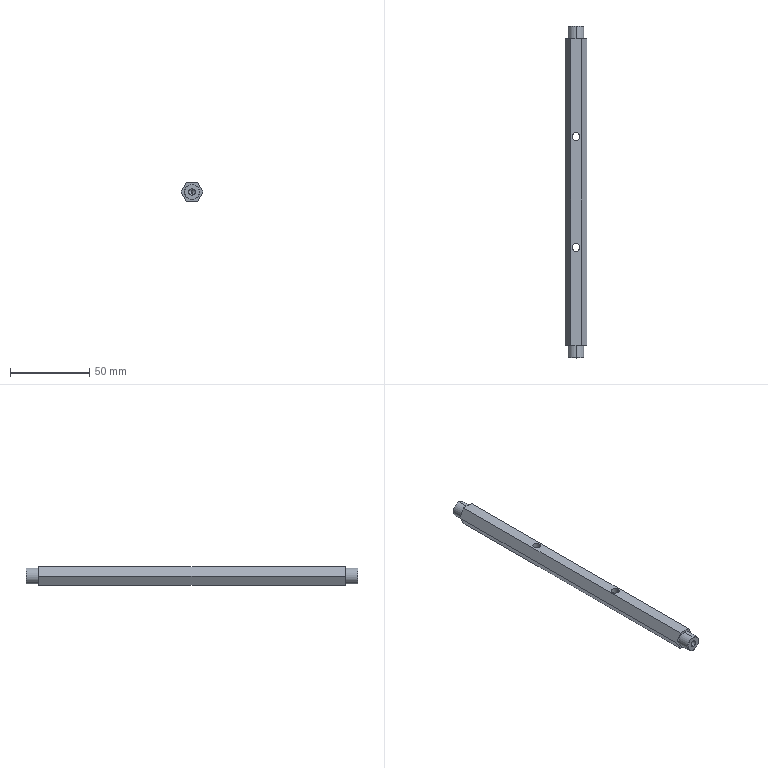Part | SolidWorks | features HoleWzd 3, ICE 2, Chamfer 1, Extrusion 1 | 1 solid | 30 faces | box 13.856 x 210 x 12 mm | volume 24621 mm3 | cylinder 12 | plane 10 | cone 8 | commonest cylinder face diameters 4.2 x4 5 x4 10 x4
STEP:
#1=CARTESIAN_POINT('',(0.,210.,4.7));
#2=VERTEX_POINT('',#1);
#3=CARTESIAN_POINT('',(0.,210.,-4.7));
#4=VERTEX_POINT('',#3);
#5=CARTESIAN_POINT('',(0.,210.,0.));
#6=DIRECTION('',(0.,1.,0.));
#7=DIRECTION('',(0.,0.,1.));
#8=AXIS2_PLACEMENT_3D('',#5,#6,#7);
#9=CIRCLE('',#8,4.7);
#10=EDGE_CURVE('',#2,#4,#9,.T.);
#11=ORIENTED_EDGE('',*,*,#10,.F.);
#12=CARTESIAN_POINT('',(0.,209.7,5.));
#13=VERTEX_POINT('',#12);
#14=CARTESIAN_POINT('',(0.,210.,4.7));
#15=DIRECTION('',(0.,-0.7071,0.7071));
#16=VECTOR('',#15,1000.);
#17=LINE('',#14,#16);
#18=EDGE_CURVE('',#2,#13,#17,.T.);
#19=ORIENTED_EDGE('',*,*,#18,.T.);
#20=CARTESIAN_POINT('',(0.,209.7,-5.));
#21=VERTEX_POINT('',#20);
#22=CARTESIAN_POINT('',(0.,209.7,0.));
#23=DIRECTION('',(0.,-1.,0.));
#24=DIRECTION('',(0.,0.,1.));
#25=AXIS2_PLACEMENT_3D('',#22,#23,#24);
#26=CIRCLE('',#25,5.);
#27=EDGE_CURVE('',#21,#13,#26,.T.);
#28=ORIENTED_EDGE('',*,*,#27,.F.);
#29=CARTESIAN_POINT('',(0.,210.,-4.7));
#30=DIRECTION('',(0.,-0.7071,-0.7071));
#31=VECTOR('',#30,1000.);
#32=LINE('',#29,#31);
#33=EDGE_CURVE('',#4,#21,#32,.T.);
#34=ORIENTED_EDGE('',*,*,#33,.F.);
#35=EDGE_LOOP('',(#11,#19,#28,#34));
#36=FACE_OUTER_BOUND('',#35,.T.);
#37=CARTESIAN_POINT('',(0.,210.,0.));
#38=DIRECTION('',(0.,-1.,0.));
#39=DIRECTION('',(0.,0.,-1.));
#40=AXIS2_PLACEMENT_3D('',#37,#38,#39);
#41=CONICAL_SURFACE('',#40,4.7,0.7854);
#42=ADVANCED_FACE('',(#36),#41,.T.);
#43=CARTESIAN_POINT('',(0.,0.,-4.7));
#44=VERTEX_POINT('',#43);
#45=CARTESIAN_POINT('',(0.,0.,4.7));
#46=VERTEX_POINT('',#45);
#47=CARTESIAN_POINT('',(0.,0.,0.));
#48=DIRECTION('',(0.,-1.,0.));
#49=DIRECTION('',(0.,0.,1.));
#50=AXIS2_PLACEMENT_3D('',#47,#48,#49);
#51=CIRCLE('',#50,4.7);
#52=EDGE_CURVE('',#44,#46,#51,.T.);
#53=ORIENTED_EDGE('',*,*,#52,.F.);
#54=CARTESIAN_POINT('',(0.,0.3,-5.));
#55=VERTEX_POINT('',#54);
#56=CARTESIAN_POINT('',(0.,0.,-4.7));
#57=DIRECTION('',(0.,0.7071,-0.7071));
#58=VECTOR('',#57,1000.);
#59=LINE('',#56,#58);
#60=EDGE_CURVE('',#44,#55,#59,.T.);
#61=ORIENTED_EDGE('',*,*,#60,.T.);
#62=CARTESIAN_POINT('',(0.,0.3,5.));
#63=VERTEX_POINT('',#62);
#64=CARTESIAN_POINT('',(0.,0.3,0.));
#65=DIRECTION('',(0.,1.,0.));
#66=DIRECTION('',(0.,0.,1.));
#67=AXIS2_PLACEMENT_3D('',#64,#65,#66);
#68=CIRCLE('',#67,5.);
#69=EDGE_CURVE('',#63,#55,#68,.T.);
#70=ORIENTED_EDGE('',*,*,#69,.F.);
#71=CARTESIAN_POINT('',(0.,0.,4.7));
#72=DIRECTION('',(0.,0.7071,0.7071));
#73=VECTOR('',#72,1000.);
#74=LINE('',#71,#73);
#75=EDGE_CURVE('',#46,#63,#74,.T.);
#76=ORIENTED_EDGE('',*,*,#75,.F.);
#77=EDGE_LOOP('',(#53,#61,#70,#76));
#78=FACE_OUTER_BOUND('',#77,.T.);
#79=CARTESIAN_POINT('',(0.,0.,0.));
#80=DIRECTION('',(0.,1.,0.));
#81=DIRECTION('',(0.,0.,1.));
#82=AXIS2_PLACEMENT_3D('',#79,#80,#81);
#83=CONICAL_SURFACE('',#82,4.7,0.7854);
#84=ADVANCED_FACE('',(#78),#83,.T.);
#85=CARTESIAN_POINT('',(0.,197.6,-2.1));
#86=VERTEX_POINT('',#85);
#87=CARTESIAN_POINT('',(0.,197.6,2.1));
#88=VERTEX_POINT('',#87);
#89=CARTESIAN_POINT('',(0.,197.6,0.));
#90=DIRECTION('',(0.,1.,0.));
#91=DIRECTION('',(0.,0.,1.));
#92=AXIS2_PLACEMENT_3D('',#89,#90,#91);
#93=CIRCLE('',#92,2.1);
#94=EDGE_CURVE('',#86,#88,#93,.T.);
#95=ORIENTED_EDGE('',*,*,#94,.F.);
#96=CARTESIAN_POINT('',(0.,210.,-2.1));
#97=VERTEX_POINT('',#96);
#98=CARTESIAN_POINT('',(0.,210.,-2.1));
#99=DIRECTION('',(0.,1.,0.));
#100=VECTOR('',#99,1000.);
#101=LINE('',#98,#100);
#102=EDGE_CURVE('',#86,#97,#101,.T.);
#103=ORIENTED_EDGE('',*,*,#102,.T.);
#104=CARTESIAN_POINT('',(0.,210.,2.1));
#105=VERTEX_POINT('',#104);
#106=CARTESIAN_POINT('',(0.,210.,0.));
#107=DIRECTION('',(0.,1.,0.));
#108=DIRECTION('',(0.,0.,1.));
#109=AXIS2_PLACEMENT_3D('',#106,#107,#108);
#110=CIRCLE('',#109,2.1);
#111=EDGE_CURVE('',#97,#105,#110,.T.);
#112=ORIENTED_EDGE('',*,*,#111,.T.);
#113=CARTESIAN_POINT('',(0.,210.,2.1));
#114=DIRECTION('',(0.,1.,0.));
#115=VECTOR('',#114,1000.);
#116=LINE('',#113,#115);
#117=EDGE_CURVE('',#88,#105,#116,.T.);
#118=ORIENTED_EDGE('',*,*,#117,.F.);
#119=EDGE_LOOP('',(#95,#103,#112,#118));
#120=FACE_OUTER_BOUND('',#119,.T.);
#121=CARTESIAN_POINT('',(0.,210.,0.));
#122=DIRECTION('',(0.,1.,0.));
#123=DIRECTION('',(0.,0.,1.));
#124=AXIS2_PLACEMENT_3D('',#121,#122,#123);
#125=CYLINDRICAL_SURFACE('',#124,2.1);
#126=ADVANCED_FACE('',(#120),#125,.F.);
#127=CARTESIAN_POINT('',(0.,196.338,0.));
#128=VERTEX_POINT('',#127);
#129=CARTESIAN_POINT('',(0.,197.6,2.1));
#130=DIRECTION('',(0.,0.515,0.8572));
#131=VECTOR('',#130,1000.);
#132=LINE('',#129,#131);
#133=EDGE_CURVE('',#128,#88,#132,.T.);
#134=ORIENTED_EDGE('',*,*,#133,.F.);
#135=CARTESIAN_POINT('',(0.,197.6,-2.1));
#136=DIRECTION('',(0.,0.515,-0.8572));
#137=VECTOR('',#136,1000.);
#138=LINE('',#135,#137);
#139=EDGE_CURVE('',#128,#86,#138,.T.);
#140=ORIENTED_EDGE('',*,*,#139,.T.);
#141=ORIENTED_EDGE('',*,*,#94,.T.);
#142=EDGE_LOOP('',(#134,#140,#141));
#143=FACE_OUTER_BOUND('',#142,.T.);
#144=CARTESIAN_POINT('',(0.,197.6,0.));
#145=DIRECTION('',(0.,1.,0.));
#146=DIRECTION('',(0.,0.,1.));
#147=AXIS2_PLACEMENT_3D('',#144,#145,#146);
#148=CONICAL_SURFACE('',#147,2.1,1.03);
#149=ADVANCED_FACE('',(#143),#148,.F.);
#150=CARTESIAN_POINT('',(0.,12.4,2.1));
#151=VERTEX_POINT('',#150);
#152=CARTESIAN_POINT('',(0.,12.4,-2.1));
#153=VERTEX_POINT('',#152);
#154=CARTESIAN_POINT('',(0.,12.4,0.));
#155=DIRECTION('',(0.,-1.,0.));
#156=DIRECTION('',(0.,0.,-1.));
#157=AXIS2_PLACEMENT_3D('',#154,#155,#156);
#158=CIRCLE('',#157,2.1);
#159=EDGE_CURVE('',#151,#153,#158,.T.);
#160=ORIENTED_EDGE('',*,*,#159,.F.);
#161=CARTESIAN_POINT('',(0.,0.,2.1));
#162=VERTEX_POINT('',#161);
#163=CARTESIAN_POINT('',(0.,0.,2.1));
#164=DIRECTION('',(0.,-1.,0.));
#165=VECTOR('',#164,1000.);
#166=LINE('',#163,#165);
#167=EDGE_CURVE('',#151,#162,#166,.T.);
#168=ORIENTED_EDGE('',*,*,#167,.T.);
#169=CARTESIAN_POINT('',(0.,0.,-2.1));
#170=VERTEX_POINT('',#169);
#171=CARTESIAN_POINT('',(0.,0.,0.));
#172=DIRECTION('',(0.,-1.,0.));
#173=DIRECTION('',(0.,0.,-1.));
#174=AXIS2_PLACEMENT_3D('',#171,#172,#173);
#175=CIRCLE('',#174,2.1);
#176=EDGE_CURVE('',#162,#170,#175,.T.);
#177=ORIENTED_EDGE('',*,*,#176,.T.);
#178=CARTESIAN_POINT('',(0.,0.,-2.1));
#179=DIRECTION('',(0.,-1.,0.));
#180=VECTOR('',#179,1000.);
#181=LINE('',#178,#180);
#182=EDGE_CURVE('',#153,#170,#181,.T.);
#183=ORIENTED_EDGE('',*,*,#182,.F.);
#184=EDGE_LOOP('',(#160,#168,#177,#183));
#185=FACE_OUTER_BOUND('',#184,.T.);
#186=CARTESIAN_POINT('',(0.,0.,0.));
#187=DIRECTION('',(0.,-1.,0.));
#188=DIRECTION('',(0.,0.,-1.));
#189=AXIS2_PLACEMENT_3D('',#186,#187,#188);
#190=CYLINDRICAL_SURFACE('',#189,2.1);
#191=ADVANCED_FACE('',(#185),#190,.F.);
#192=CARTESIAN_POINT('',(0.,13.662,0.));
#193=VERTEX_POINT('',#192);
#194=CARTESIAN_POINT('',(0.,12.4,-2.1));
#195=DIRECTION('',(0.,-0.515,-0.8572));
#196=VECTOR('',#195,1000.);
#197=LINE('',#194,#196);
#198=EDGE_CURVE('',#193,#153,#197,.T.);
#199=ORIENTED_EDGE('',*,*,#198,.F.);
#200=CARTESIAN_POINT('',(0.,12.4,2.1));
#201=DIRECTION('',(0.,-0.515,0.8572));
#202=VECTOR('',#201,1000.);
#203=LINE('',#200,#202);
#204=EDGE_CURVE('',#193,#151,#203,.T.);
#205=ORIENTED_EDGE('',*,*,#204,.T.);
#206=ORIENTED_EDGE('',*,*,#159,.T.);
#207=EDGE_LOOP('',(#199,#205,#206));
#208=FACE_OUTER_BOUND('',#207,.T.);
#209=CARTESIAN_POINT('',(0.,12.4,0.));
#210=DIRECTION('',(0.,-1.,0.));
#211=DIRECTION('',(0.,0.,-1.));
#212=AXIS2_PLACEMENT_3D('',#209,#210,#211);
#213=CONICAL_SURFACE('',#212,2.1,1.03);
#214=ADVANCED_FACE('',(#208),#213,.F.);
#215=CARTESIAN_POINT('',(2.5,140.,6.));
#216=VERTEX_POINT('',#215);
#217=CARTESIAN_POINT('',(-2.5,140.,6.));
#218=VERTEX_POINT('',#217);
#219=CARTESIAN_POINT('',(0.,140.,6.));
#220=DIRECTION('',(0.,0.,-1.));
#221=DIRECTION('',(-1.,0.,0.));
#222=AXIS2_PLACEMENT_3D('',#219,#220,#221);
#223=CIRCLE('',#222,2.5);
#224=EDGE_CURVE('',#216,#218,#223,.T.);
#225=ORIENTED_EDGE('',*,*,#224,.F.);
#226=CARTESIAN_POINT('',(2.5,140.,-6.));
#227=VERTEX_POINT('',#226);
#228=CARTESIAN_POINT('',(2.5,140.,-6.));
#229=DIRECTION('',(0.,0.,-1.));
#230=VECTOR('',#229,1000.);
#231=LINE('',#228,#230);
#232=EDGE_CURVE('',#216,#227,#231,.T.);
#233=ORIENTED_EDGE('',*,*,#232,.T.);
#234=CARTESIAN_POINT('',(-2.5,140.,-6.));
#235=VERTEX_POINT('',#234);
#236=CARTESIAN_POINT('',(0.,140.,-6.));
#237=DIRECTION('',(0.,0.,-1.));
#238=DIRECTION('',(-1.,0.,0.));
#239=AXIS2_PLACEMENT_3D('',#236,#237,#238);
#240=CIRCLE('',#239,2.5);
#241=EDGE_CURVE('',#227,#235,#240,.T.);
#242=ORIENTED_EDGE('',*,*,#241,.T.);
#243=CARTESIAN_POINT('',(-2.5,140.,-6.));
#244=DIRECTION('',(0.,0.,-1.));
#245=VECTOR('',#244,1000.);
#246=LINE('',#243,#245);
#247=EDGE_CURVE('',#218,#235,#246,.T.);
#248=ORIENTED_EDGE('',*,*,#247,.F.);
#249=EDGE_LOOP('',(#225,#233,#242,#248));
#250=FACE_OUTER_BOUND('',#249,.T.);
#251=CARTESIAN_POINT('',(0.,140.,-6.));
#252=DIRECTION('',(0.,0.,-1.));
#253=DIRECTION('',(-1.,0.,0.));
#254=AXIS2_PLACEMENT_3D('',#251,#252,#253);
#255=CYLINDRICAL_SURFACE('',#254,2.5);
#256=ADVANCED_FACE('',(#250),#255,.F.);
#257=CARTESIAN_POINT('',(2.5,70.,6.));
#258=VERTEX_POINT('',#257);
#259=CARTESIAN_POINT('',(-2.5,70.,6.));
#260=VERTEX_POINT('',#259);
#261=CARTESIAN_POINT('',(0.,70.,6.));
#262=DIRECTION('',(0.,0.,-1.));
#263=DIRECTION('',(-1.,0.,0.));
#264=AXIS2_PLACEMENT_3D('',#261,#262,#263);
#265=CIRCLE('',#264,2.5);
#266=EDGE_CURVE('',#258,#260,#265,.T.);
#267=ORIENTED_EDGE('',*,*,#266,.F.);
#268=CARTESIAN_POINT('',(2.5,70.,-6.));
#269=VERTEX_POINT('',#268);
#270=CARTESIAN_POINT('',(2.5,70.,-6.));
#271=DIRECTION('',(0.,0.,-1.));
#272=VECTOR('',#271,1000.);
#273=LINE('',#270,#272);
#274=EDGE_CURVE('',#258,#269,#273,.T.);
#275=ORIENTED_EDGE('',*,*,#274,.T.);
#276=CARTESIAN_POINT('',(-2.5,70.,-6.));
#277=VERTEX_POINT('',#276);
#278=CARTESIAN_POINT('',(0.,70.,-6.));
#279=DIRECTION('',(0.,0.,-1.));
#280=DIRECTION('',(-1.,0.,0.));
#281=AXIS2_PLACEMENT_3D('',#278,#279,#280);
#282=CIRCLE('',#281,2.5);
#283=EDGE_CURVE('',#269,#277,#282,.T.);
#284=ORIENTED_EDGE('',*,*,#283,.T.);
#285=CARTESIAN_POINT('',(-2.5,70.,-6.));
#286=DIRECTION('',(0.,0.,-1.));
#287=VECTOR('',#286,1000.);
#288=LINE('',#285,#287);
#289=EDGE_CURVE('',#260,#277,#288,.T.);
#290=ORIENTED_EDGE('',*,*,#289,.F.);
#291=EDGE_LOOP('',(#267,#275,#284,#290));
#292=FACE_OUTER_BOUND('',#291,.T.);
#293=CARTESIAN_POINT('',(0.,70.,-6.));
#294=DIRECTION('',(0.,0.,-1.));
#295=DIRECTION('',(-1.,0.,0.));
#296=AXIS2_PLACEMENT_3D('',#293,#294,#295);
#297=CYLINDRICAL_SURFACE('',#296,2.5);
#298=ADVANCED_FACE('',(#292),#297,.F.);
#299=CARTESIAN_POINT('',(0.,8.,-5.));
#300=VERTEX_POINT('',#299);
#301=CARTESIAN_POINT('',(0.,8.,5.));
#302=VERTEX_POINT('',#301);
#303=CARTESIAN_POINT('',(0.,8.,0.));
#304=DIRECTION('',(0.,-1.,0.));
#305=DIRECTION('',(0.,0.,-1.));
#306=AXIS2_PLACEMENT_3D('',#303,#304,#305);
#307=CIRCLE('',#306,5.);
#308=EDGE_CURVE('',#300,#302,#307,.T.);
#309=ORIENTED_EDGE('',*,*,#308,.T.);
#310=CARTESIAN_POINT('',(0.,8.,5.));
#311=DIRECTION('',(0.,-1.,0.));
#312=VECTOR('',#311,1000.);
#313=LINE('',#310,#312);
#314=EDGE_CURVE('',#302,#63,#313,.T.);
#315=ORIENTED_EDGE('',*,*,#314,.T.);
#316=ORIENTED_EDGE('',*,*,#69,.T.);
#317=CARTESIAN_POINT('',(0.,8.,-5.));
#318=DIRECTION('',(0.,-1.,0.));
#319=VECTOR('',#318,1000.);
#320=LINE('',#317,#319);
#321=EDGE_CURVE('',#300,#55,#320,.T.);
#322=ORIENTED_EDGE('',*,*,#321,.F.);
#323=EDGE_LOOP('',(#309,#315,#316,#322));
#324=FACE_OUTER_BOUND('',#323,.T.);
#325=CARTESIAN_POINT('',(0.,8.,0.));
#326=DIRECTION('',(0.,-1.,0.));
#327=DIRECTION('',(0.,0.,-1.));
#328=AXIS2_PLACEMENT_3D('',#325,#326,#327);
#329=CYLINDRICAL_SURFACE('',#328,5.);
#330=ADVANCED_FACE('',(#324),#329,.T.);
#331=CARTESIAN_POINT('',(0.,202.,5.));
#332=VERTEX_POINT('',#331);
#333=CARTESIAN_POINT('',(0.,202.,-5.));
#334=VERTEX_POINT('',#333);
#335=CARTESIAN_POINT('',(0.,202.,0.));
#336=DIRECTION('',(0.,1.,0.));
#337=DIRECTION('',(0.,0.,1.));
#338=AXIS2_PLACEMENT_3D('',#335,#336,#337);
#339=CIRCLE('',#338,5.);
#340=EDGE_CURVE('',#332,#334,#339,.T.);
#341=ORIENTED_EDGE('',*,*,#340,.T.);
#342=CARTESIAN_POINT('',(0.,202.,-5.));
#343=DIRECTION('',(0.,1.,0.));
#344=VECTOR('',#343,1000.);
#345=LINE('',#342,#344);
#346=EDGE_CURVE('',#334,#21,#345,.T.);
#347=ORIENTED_EDGE('',*,*,#346,.T.);
#348=ORIENTED_EDGE('',*,*,#27,.T.);
#349=CARTESIAN_POINT('',(0.,202.,5.));
#350=DIRECTION('',(0.,1.,0.));
#351=VECTOR('',#350,1000.);
#352=LINE('',#349,#351);
#353=EDGE_CURVE('',#332,#13,#352,.T.);
#354=ORIENTED_EDGE('',*,*,#353,.F.);
#355=EDGE_LOOP('',(#341,#347,#348,#354));
#356=FACE_OUTER_BOUND('',#355,.T.);
#357=CARTESIAN_POINT('',(0.,202.,0.));
#358=DIRECTION('',(0.,1.,0.));
#359=DIRECTION('',(0.,0.,1.));
#360=AXIS2_PLACEMENT_3D('',#357,#358,#359);
#361=CYLINDRICAL_SURFACE('',#360,5.);
#362=ADVANCED_FACE('',(#356),#361,.T.);
#363=CARTESIAN_POINT('',(6.928,8.,0.));
#364=VERTEX_POINT('',#363);
#365=CARTESIAN_POINT('',(3.464,8.,6.));
#366=VERTEX_POINT('',#365);
#367=CARTESIAN_POINT('',(3.464,8.,6.));
#368=DIRECTION('',(-0.5,0.,0.866));
#369=VECTOR('',#368,1000.);
#370=LINE('',#367,#369);
#371=EDGE_CURVE('',#364,#366,#370,.T.);
#372=ORIENTED_EDGE('',*,*,#371,.F.);
#373=CARTESIAN_POINT('',(6.928,202.,0.));
#374=VERTEX_POINT('',#373);
#375=CARTESIAN_POINT('',(6.928,210.,0.));
#376=DIRECTION('',(0.,-1.,0.));
#377=VECTOR('',#376,1000.);
#378=LINE('',#375,#377);
#379=EDGE_CURVE('',#374,#364,#378,.T.);
#380=ORIENTED_EDGE('',*,*,#379,.F.);
#381=CARTESIAN_POINT('',(3.464,202.,6.));
#382=VERTEX_POINT('',#381);
#383=CARTESIAN_POINT('',(3.464,202.,6.));
#384=DIRECTION('',(0.5,0.,-0.866));
#385=VECTOR('',#384,1000.);
#386=LINE('',#383,#385);
#387=EDGE_CURVE('',#382,#374,#386,.T.);
#388=ORIENTED_EDGE('',*,*,#387,.F.);
#389=CARTESIAN_POINT('',(3.464,210.,6.));
#390=DIRECTION('',(0.,-1.,0.));
#391=VECTOR('',#390,1000.);
#392=LINE('',#389,#391);
#393=EDGE_CURVE('',#382,#366,#392,.T.);
#394=ORIENTED_EDGE('',*,*,#393,.T.);
#395=EDGE_LOOP('',(#372,#380,#388,#394));
#396=FACE_OUTER_BOUND('',#395,.T.);
#397=CARTESIAN_POINT('',(3.464,210.,6.));
#398=DIRECTION('',(-0.866,0.,-0.5));
#399=DIRECTION('',(-0.5,0.,0.866));
#400=AXIS2_PLACEMENT_3D('',#397,#398,#399);
#401=PLANE('',#400);
#402=ADVANCED_FACE('',(#396),#401,.F.);
#403=CARTESIAN_POINT('',(3.464,8.,-6.));
#404=VERTEX_POINT('',#403);
#405=CARTESIAN_POINT('',(6.928,8.,0.));
#406=DIRECTION('',(0.5,0.,0.866));
#407=VECTOR('',#406,1000.);
#408=LINE('',#405,#407);
#409=EDGE_CURVE('',#404,#364,#408,.T.);
#410=ORIENTED_EDGE('',*,*,#409,.F.);
#411=CARTESIAN_POINT('',(3.464,202.,-6.));
#412=VERTEX_POINT('',#411);
#413=CARTESIAN_POINT('',(3.464,210.,-6.));
#414=DIRECTION('',(0.,-1.,0.));
#415=VECTOR('',#414,1000.);
#416=LINE('',#413,#415);
#417=EDGE_CURVE('',#412,#404,#416,.T.);
#418=ORIENTED_EDGE('',*,*,#417,.F.);
#419=CARTESIAN_POINT('',(6.928,202.,0.));
#420=DIRECTION('',(-0.5,0.,-0.866));
#421=VECTOR('',#420,1000.);
#422=LINE('',#419,#421);
#423=EDGE_CURVE('',#374,#412,#422,.T.);
#424=ORIENTED_EDGE('',*,*,#423,.F.);
#425=ORIENTED_EDGE('',*,*,#379,.T.);
#426=EDGE_LOOP('',(#410,#418,#424,#425));
#427=FACE_OUTER_BOUND('',#426,.T.);
#428=CARTESIAN_POINT('',(6.928,210.,0.));
#429=DIRECTION('',(-0.866,0.,0.5));
#430=DIRECTION('',(0.5,0.,0.866));
#431=AXIS2_PLACEMENT_3D('',#428,#429,#430);
#432=PLANE('',#431);
#433=ADVANCED_FACE('',(#427),#432,.F.);
#434=CARTESIAN_POINT('',(0.,140.,-6.));
#435=DIRECTION('',(0.,0.,-1.));
#436=DIRECTION('',(-1.,0.,0.));
#437=AXIS2_PLACEMENT_3D('',#434,#435,#436);
#438=CIRCLE('',#437,2.5);
#439=EDGE_CURVE('',#235,#227,#438,.T.);
#440=ORIENTED_EDGE('',*,*,#439,.F.);
#441=ORIENTED_EDGE('',*,*,#241,.F.);
#442=EDGE_LOOP('',(#440,#441));
#443=FACE_BOUND('',#442,.T.);
#444=CARTESIAN_POINT('',(0.,70.,-6.));
#445=DIRECTION('',(0.,0.,-1.));
#446=DIRECTION('',(-1.,0.,0.));
#447=AXIS2_PLACEMENT_3D('',#444,#445,#446);
#448=CIRCLE('',#447,2.5);
#449=EDGE_CURVE('',#277,#269,#448,.T.);
#450=ORIENTED_EDGE('',*,*,#449,.F.);
#451=ORIENTED_EDGE('',*,*,#283,.F.);
#452=EDGE_LOOP('',(#450,#451));
#453=FACE_BOUND('',#452,.T.);
#454=CARTESIAN_POINT('',(-3.464,8.,-6.));
#455=VERTEX_POINT('',#454);
#456=CARTESIAN_POINT('',(3.464,8.,-6.));
#457=DIRECTION('',(1.,0.,0.));
#458=VECTOR('',#457,1000.);
#459=LINE('',#456,#458);
#460=EDGE_CURVE('',#455,#404,#459,.T.);
#461=ORIENTED_EDGE('',*,*,#460,.F.);
#462=CARTESIAN_POINT('',(-3.464,202.,-6.));
#463=VERTEX_POINT('',#462);
#464=CARTESIAN_POINT('',(-3.464,210.,-6.));
#465=DIRECTION('',(0.,-1.,0.));
#466=VECTOR('',#465,1000.);
#467=LINE('',#464,#466);
#468=EDGE_CURVE('',#463,#455,#467,.T.);
#469=ORIENTED_EDGE('',*,*,#468,.F.);
#470=CARTESIAN_POINT('',(3.464,202.,-6.));
#471=DIRECTION('',(-1.,0.,0.));
#472=VECTOR('',#471,1000.);
#473=LINE('',#470,#472);
#474=EDGE_CURVE('',#412,#463,#473,.T.);
#475=ORIENTED_EDGE('',*,*,#474,.F.);
#476=ORIENTED_EDGE('',*,*,#417,.T.);
#477=EDGE_LOOP('',(#461,#469,#475,#476));
#478=FACE_OUTER_BOUND('',#477,.T.);
#479=CARTESIAN_POINT('',(3.464,210.,-6.));
#480=DIRECTION('',(0.,0.,1.));
#481=DIRECTION('',(1.,0.,0.));
#482=AXIS2_PLACEMENT_3D('',#479,#480,#481);
#483=PLANE('',#482);
#484=ADVANCED_FACE('',(#443,#453,#478),#483,.F.);
#485=CARTESIAN_POINT('',(-6.928,8.,0.));
#486=VERTEX_POINT('',#485);
#487=CARTESIAN_POINT('',(-3.464,8.,-6.));
#488=DIRECTION('',(0.5,0.,-0.866));
#489=VECTOR('',#488,1000.);
#490=LINE('',#487,#489);
#491=EDGE_CURVE('',#486,#455,#490,.T.);
#492=ORIENTED_EDGE('',*,*,#491,.F.);
#493=CARTESIAN_POINT('',(-6.928,202.,0.));
#494=VERTEX_POINT('',#493);
#495=CARTESIAN_POINT('',(-6.928,210.,0.));
#496=DIRECTION('',(0.,-1.,0.));
#497=VECTOR('',#496,1000.);
#498=LINE('',#495,#497);
#499=EDGE_CURVE('',#494,#486,#498,.T.);
#500=ORIENTED_EDGE('',*,*,#499,.F.);
#501=CARTESIAN_POINT('',(-3.464,202.,-6.));
#502=DIRECTION('',(-0.5,0.,0.866));
#503=VECTOR('',#502,1000.);
#504=LINE('',#501,#503);
#505=EDGE_CURVE('',#463,#494,#504,.T.);
#506=ORIENTED_EDGE('',*,*,#505,.F.);
#507=ORIENTED_EDGE('',*,*,#468,.T.);
#508=EDGE_LOOP('',(#492,#500,#506,#507));
#509=FACE_OUTER_BOUND('',#508,.T.);
#510=CARTESIAN_POINT('',(-3.464,210.,-6.));
#511=DIRECTION('',(0.866,0.,0.5));
#512=DIRECTION('',(0.5,0.,-0.866));
#513=AXIS2_PLACEMENT_3D('',#510,#511,#512);
#514=PLANE('',#513);
#515=ADVANCED_FACE('',(#509),#514,.F.);
#516=CARTESIAN_POINT('',(-3.464,8.,6.));
#517=VERTEX_POINT('',#516);
#518=CARTESIAN_POINT('',(-6.928,8.,0.));
#519=DIRECTION('',(-0.5,0.,-0.866));
#520=VECTOR('',#519,1000.);
#521=LINE('',#518,#520);
#522=EDGE_CURVE('',#517,#486,#521,.T.);
#523=ORIENTED_EDGE('',*,*,#522,.F.);
#524=CARTESIAN_POINT('',(-3.464,202.,6.));
#525=VERTEX_POINT('',#524);
#526=CARTESIAN_POINT('',(-3.464,210.,6.));
#527=DIRECTION('',(0.,-1.,0.));
#528=VECTOR('',#527,1000.);
#529=LINE('',#526,#528);
#530=EDGE_CURVE('',#525,#517,#529,.T.);
#531=ORIENTED_EDGE('',*,*,#530,.F.);
#532=CARTESIAN_POINT('',(-6.928,202.,0.));
#533=DIRECTION('',(0.5,0.,0.866));
#534=VECTOR('',#533,1000.);
#535=LINE('',#532,#534);
#536=EDGE_CURVE('',#494,#525,#535,.T.);
#537=ORIENTED_EDGE('',*,*,#536,.F.);
#538=ORIENTED_EDGE('',*,*,#499,.T.);
#539=EDGE_LOOP('',(#523,#531,#537,#538));
#540=FACE_OUTER_BOUND('',#539,.T.);
#541=CARTESIAN_POINT('',(-6.928,210.,0.));
#542=DIRECTION('',(0.866,0.,-0.5));
#543=DIRECTION('',(-0.5,0.,-0.866));
#544=AXIS2_PLACEMENT_3D('',#541,#542,#543);
#545=PLANE('',#544);
#546=ADVANCED_FACE('',(#540),#545,.F.);
#547=CARTESIAN_POINT('',(0.,140.,6.));
#548=DIRECTION('',(0.,0.,-1.));
#549=DIRECTION('',(-1.,0.,0.));
#550=AXIS2_PLACEMENT_3D('',#547,#548,#549);
#551=CIRCLE('',#550,2.5);
#552=EDGE_CURVE('',#218,#216,#551,.T.);
#553=ORIENTED_EDGE('',*,*,#552,.T.);
#554=ORIENTED_EDGE('',*,*,#224,.T.);
#555=EDGE_LOOP('',(#553,#554));
#556=FACE_BOUND('',#555,.T.);
#557=CARTESIAN_POINT('',(0.,70.,6.));
#558=DIRECTION('',(0.,0.,-1.));
#559=DIRECTION('',(-1.,0.,0.));
#560=AXIS2_PLACEMENT_3D('',#557,#558,#559);
#561=CIRCLE('',#560,2.5);
#562=EDGE_CURVE('',#260,#258,#561,.T.);
#563=ORIENTED_EDGE('',*,*,#562,.T.);
#564=ORIENTED_EDGE('',*,*,#266,.T.);
#565=EDGE_LOOP('',(#563,#564));
#566=FACE_BOUND('',#565,.T.);
#567=CARTESIAN_POINT('',(-3.464,8.,6.));
#568=DIRECTION('',(-1.,0.,0.));
#569=VECTOR('',#568,1000.);
#570=LINE('',#567,#569);
#571=EDGE_CURVE('',#366,#517,#570,.T.);
#572=ORIENTED_EDGE('',*,*,#571,.F.);
#573=ORIENTED_EDGE('',*,*,#393,.F.);
#574=CARTESIAN_POINT('',(-3.464,202.,6.));
#575=DIRECTION('',(1.,0.,0.));
#576=VECTOR('',#575,1000.);
#577=LINE('',#574,#576);
#578=EDGE_CURVE('',#525,#382,#577,.T.);
#579=ORIENTED_EDGE('',*,*,#578,.F.);
#580=ORIENTED_EDGE('',*,*,#530,.T.);
#581=EDGE_LOOP('',(#572,#573,#579,#580));
#582=FACE_OUTER_BOUND('',#581,.T.);
#583=CARTESIAN_POINT('',(-3.464,210.,6.));
#584=DIRECTION('',(0.,0.,-1.));
#585=DIRECTION('',(-1.,0.,0.));
#586=AXIS2_PLACEMENT_3D('',#583,#584,#585);
#587=PLANE('',#586);
#588=ADVANCED_FACE('',(#556,#566,#582),#587,.F.);
#589=ORIENTED_EDGE('',*,*,#340,.F.);
#590=CARTESIAN_POINT('',(0.,202.,0.));
#591=DIRECTION('',(0.,1.,0.));
#592=DIRECTION('',(0.,0.,1.));
#593=AXIS2_PLACEMENT_3D('',#590,#591,#592);
#594=CIRCLE('',#593,5.);
#595=EDGE_CURVE('',#334,#332,#594,.T.);
#596=ORIENTED_EDGE('',*,*,#595,.F.);
#597=EDGE_LOOP('',(#589,#596));
#598=FACE_BOUND('',#597,.T.);
#599=ORIENTED_EDGE('',*,*,#387,.T.);
#600=ORIENTED_EDGE('',*,*,#423,.T.);
#601=ORIENTED_EDGE('',*,*,#474,.T.);
#602=ORIENTED_EDGE('',*,*,#505,.T.);
#603=ORIENTED_EDGE('',*,*,#536,.T.);
#604=ORIENTED_EDGE('',*,*,#578,.T.);
#605=EDGE_LOOP('',(#599,#600,#601,#602,#603,#604));
#606=FACE_OUTER_BOUND('',#605,.T.);
#607=CARTESIAN_POINT('',(0.,202.,0.));
#608=DIRECTION('',(0.,1.,0.));
#609=DIRECTION('',(0.,0.,1.));
#610=AXIS2_PLACEMENT_3D('',#607,#608,#609);
#611=PLANE('',#610);
#612=ADVANCED_FACE('',(#598,#606),#611,.T.);
#613=ORIENTED_EDGE('',*,*,#346,.F.);
#614=ORIENTED_EDGE('',*,*,#595,.T.);
#615=ORIENTED_EDGE('',*,*,#353,.T.);
#616=CARTESIAN_POINT('',(0.,209.7,0.));
#617=DIRECTION('',(0.,-1.,0.));
#618=DIRECTION('',(0.,0.,1.));
#619=AXIS2_PLACEMENT_3D('',#616,#617,#618);
#620=CIRCLE('',#619,5.);
#621=EDGE_CURVE('',#13,#21,#620,.T.);
#622=ORIENTED_EDGE('',*,*,#621,.T.);
#623=EDGE_LOOP('',(#613,#614,#615,#622));
#624=FACE_OUTER_BOUND('',#623,.T.);
#625=CARTESIAN_POINT('',(0.,202.,0.));
#626=DIRECTION('',(0.,1.,0.));
#627=DIRECTION('',(0.,0.,1.));
#628=AXIS2_PLACEMENT_3D('',#625,#626,#627);
#629=CYLINDRICAL_SURFACE('',#628,5.);
#630=ADVANCED_FACE('',(#624),#629,.T.);
#631=CARTESIAN_POINT('',(0.,210.,0.));
#632=DIRECTION('',(0.,1.,0.));
#633=DIRECTION('',(0.,0.,1.));
#634=AXIS2_PLACEMENT_3D('',#631,#632,#633);
#635=CIRCLE('',#634,4.7);
#636=EDGE_CURVE('',#4,#2,#635,.T.);
#637=ORIENTED_EDGE('',*,*,#636,.T.);
#638=ORIENTED_EDGE('',*,*,#10,.T.);
#639=EDGE_LOOP('',(#637,#638));
#640=FACE_OUTER_BOUND('',#639,.T.);
#641=CARTESIAN_POINT('',(0.,210.,0.));
#642=DIRECTION('',(0.,1.,0.));
#643=DIRECTION('',(0.,0.,1.));
#644=AXIS2_PLACEMENT_3D('',#641,#642,#643);
#645=CIRCLE('',#644,2.1);
#646=EDGE_CURVE('',#105,#97,#645,.T.);
#647=ORIENTED_EDGE('',*,*,#646,.F.);
#648=ORIENTED_EDGE('',*,*,#111,.F.);
#649=EDGE_LOOP('',(#647,#648));
#650=FACE_BOUND('',#649,.T.);
#651=CARTESIAN_POINT('',(6.928,210.,0.));
#652=DIRECTION('',(0.,1.,0.));
#653=DIRECTION('',(0.,0.,1.));
#654=AXIS2_PLACEMENT_3D('',#651,#652,#653);
#655=PLANE('',#654);
#656=ADVANCED_FACE('',(#640,#650),#655,.T.);
#657=ORIENTED_EDGE('',*,*,#308,.F.);
#658=CARTESIAN_POINT('',(0.,8.,0.));
#659=DIRECTION('',(0.,-1.,0.));
#660=DIRECTION('',(0.,0.,-1.));
#661=AXIS2_PLACEMENT_3D('',#658,#659,#660);
#662=CIRCLE('',#661,5.);
#663=EDGE_CURVE('',#302,#300,#662,.T.);
#664=ORIENTED_EDGE('',*,*,#663,.F.);
#665=EDGE_LOOP('',(#657,#664));
#666=FACE_BOUND('',#665,.T.);
#667=ORIENTED_EDGE('',*,*,#371,.T.);
#668=ORIENTED_EDGE('',*,*,#571,.T.);
#669=ORIENTED_EDGE('',*,*,#522,.T.);
#670=ORIENTED_EDGE('',*,*,#491,.T.);
#671=ORIENTED_EDGE('',*,*,#460,.T.);
#672=ORIENTED_EDGE('',*,*,#409,.T.);
#673=EDGE_LOOP('',(#667,#668,#669,#670,#671,#672));
#674=FACE_OUTER_BOUND('',#673,.T.);
#675=CARTESIAN_POINT('',(0.,8.,0.));
#676=DIRECTION('',(0.,-1.,0.));
#677=DIRECTION('',(0.,0.,-1.));
#678=AXIS2_PLACEMENT_3D('',#675,#676,#677);
#679=PLANE('',#678);
#680=ADVANCED_FACE('',(#666,#674),#679,.T.);
#681=ORIENTED_EDGE('',*,*,#314,.F.);
#682=ORIENTED_EDGE('',*,*,#663,.T.);
#683=ORIENTED_EDGE('',*,*,#321,.T.);
#684=CARTESIAN_POINT('',(0.,0.3,0.));
#685=DIRECTION('',(0.,1.,0.));
#686=DIRECTION('',(0.,0.,1.));
#687=AXIS2_PLACEMENT_3D('',#684,#685,#686);
#688=CIRCLE('',#687,5.);
#689=EDGE_CURVE('',#55,#63,#688,.T.);
#690=ORIENTED_EDGE('',*,*,#689,.T.);
#691=EDGE_LOOP('',(#681,#682,#683,#690));
#692=FACE_OUTER_BOUND('',#691,.T.);
#693=CARTESIAN_POINT('',(0.,8.,0.));
#694=DIRECTION('',(0.,-1.,0.));
#695=DIRECTION('',(0.,0.,-1.));
#696=AXIS2_PLACEMENT_3D('',#693,#694,#695);
#697=CYLINDRICAL_SURFACE('',#696,5.);
#698=ADVANCED_FACE('',(#692),#697,.T.);
#699=CARTESIAN_POINT('',(0.,0.,0.));
#700=DIRECTION('',(0.,-1.,0.));
#701=DIRECTION('',(0.,0.,1.));
#702=AXIS2_PLACEMENT_3D('',#699,#700,#701);
#703=CIRCLE('',#702,4.7);
#704=EDGE_CURVE('',#46,#44,#703,.T.);
#705=ORIENTED_EDGE('',*,*,#704,.T.);
#706=ORIENTED_EDGE('',*,*,#52,.T.);
#707=EDGE_LOOP('',(#705,#706));
#708=FACE_OUTER_BOUND('',#707,.T.);
#709=CARTESIAN_POINT('',(0.,0.,0.));
#710=DIRECTION('',(0.,-1.,0.));
#711=DIRECTION('',(0.,0.,-1.));
#712=AXIS2_PLACEMENT_3D('',#709,#710,#711);
#713=CIRCLE('',#712,2.1);
#714=EDGE_CURVE('',#170,#162,#713,.T.);
#715=ORIENTED_EDGE('',*,*,#714,.F.);
#716=ORIENTED_EDGE('',*,*,#176,.F.);
#717=EDGE_LOOP('',(#715,#716));
#718=FACE_BOUND('',#717,.T.);
#719=CARTESIAN_POINT('',(6.928,0.,0.));
#720=DIRECTION('',(0.,1.,0.));
#721=DIRECTION('',(0.,0.,1.));
#722=AXIS2_PLACEMENT_3D('',#719,#720,#721);
#723=PLANE('',#722);
#724=ADVANCED_FACE('',(#708,#718),#723,.F.);
#725=ORIENTED_EDGE('',*,*,#274,.F.);
#726=ORIENTED_EDGE('',*,*,#562,.F.);
#727=ORIENTED_EDGE('',*,*,#289,.T.);
#728=ORIENTED_EDGE('',*,*,#449,.T.);
#729=EDGE_LOOP('',(#725,#726,#727,#728));
#730=FACE_OUTER_BOUND('',#729,.T.);
#731=CARTESIAN_POINT('',(0.,70.,-6.));
#732=DIRECTION('',(0.,0.,-1.));
#733=DIRECTION('',(-1.,0.,0.));
#734=AXIS2_PLACEMENT_3D('',#731,#732,#733);
#735=CYLINDRICAL_SURFACE('',#734,2.5);
#736=ADVANCED_FACE('',(#730),#735,.F.);
#737=ORIENTED_EDGE('',*,*,#232,.F.);
#738=ORIENTED_EDGE('',*,*,#552,.F.);
#739=ORIENTED_EDGE('',*,*,#247,.T.);
#740=ORIENTED_EDGE('',*,*,#439,.T.);
#741=EDGE_LOOP('',(#737,#738,#739,#740));
#742=FACE_OUTER_BOUND('',#741,.T.);
#743=CARTESIAN_POINT('',(0.,140.,-6.));
#744=DIRECTION('',(0.,0.,-1.));
#745=DIRECTION('',(-1.,0.,0.));
#746=AXIS2_PLACEMENT_3D('',#743,#744,#745);
#747=CYLINDRICAL_SURFACE('',#746,2.5);
#748=ADVANCED_FACE('',(#742),#747,.F.);
#749=ORIENTED_EDGE('',*,*,#204,.F.);
#750=ORIENTED_EDGE('',*,*,#198,.T.);
#751=CARTESIAN_POINT('',(0.,12.4,0.));
#752=DIRECTION('',(0.,-1.,0.));
#753=DIRECTION('',(0.,0.,-1.));
#754=AXIS2_PLACEMENT_3D('',#751,#752,#753);
#755=CIRCLE('',#754,2.1);
#756=EDGE_CURVE('',#153,#151,#755,.T.);
#757=ORIENTED_EDGE('',*,*,#756,.T.);
#758=EDGE_LOOP('',(#749,#750,#757));
#759=FACE_OUTER_BOUND('',#758,.T.);
#760=CARTESIAN_POINT('',(0.,12.4,0.));
#761=DIRECTION('',(0.,-1.,0.));
#762=DIRECTION('',(0.,0.,-1.));
#763=AXIS2_PLACEMENT_3D('',#760,#761,#762);
#764=CONICAL_SURFACE('',#763,2.1,1.03);
#765=ADVANCED_FACE('',(#759),#764,.F.);
#766=ORIENTED_EDGE('',*,*,#167,.F.);
#767=ORIENTED_EDGE('',*,*,#756,.F.);
#768=ORIENTED_EDGE('',*,*,#182,.T.);
#769=ORIENTED_EDGE('',*,*,#714,.T.);
#770=EDGE_LOOP('',(#766,#767,#768,#769));
#771=FACE_OUTER_BOUND('',#770,.T.);
#772=CARTESIAN_POINT('',(0.,0.,0.));
#773=DIRECTION('',(0.,-1.,0.));
#774=DIRECTION('',(0.,0.,-1.));
#775=AXIS2_PLACEMENT_3D('',#772,#773,#774);
#776=CYLINDRICAL_SURFACE('',#775,2.1);
#777=ADVANCED_FACE('',(#771),#776,.F.);
#778=ORIENTED_EDGE('',*,*,#139,.F.);
#779=ORIENTED_EDGE('',*,*,#133,.T.);
#780=CARTESIAN_POINT('',(0.,197.6,0.));
#781=DIRECTION('',(0.,1.,0.));
#782=DIRECTION('',(0.,0.,1.));
#783=AXIS2_PLACEMENT_3D('',#780,#781,#782);
#784=CIRCLE('',#783,2.1);
#785=EDGE_CURVE('',#88,#86,#784,.T.);
#786=ORIENTED_EDGE('',*,*,#785,.T.);
#787=EDGE_LOOP('',(#778,#779,#786));
#788=FACE_OUTER_BOUND('',#787,.T.);
#789=CARTESIAN_POINT('',(0.,197.6,0.));
#790=DIRECTION('',(0.,1.,0.));
#791=DIRECTION('',(0.,0.,1.));
#792=AXIS2_PLACEMENT_3D('',#789,#790,#791);
#793=CONICAL_SURFACE('',#792,2.1,1.03);
#794=ADVANCED_FACE('',(#788),#793,.F.);
#795=ORIENTED_EDGE('',*,*,#102,.F.);
#796=ORIENTED_EDGE('',*,*,#785,.F.);
#797=ORIENTED_EDGE('',*,*,#117,.T.);
#798=ORIENTED_EDGE('',*,*,#646,.T.);
#799=EDGE_LOOP('',(#795,#796,#797,#798));
#800=FACE_OUTER_BOUND('',#799,.T.);
#801=CARTESIAN_POINT('',(0.,210.,0.));
#802=DIRECTION('',(0.,1.,0.));
#803=DIRECTION('',(0.,0.,1.));
#804=AXIS2_PLACEMENT_3D('',#801,#802,#803);
#805=CYLINDRICAL_SURFACE('',#804,2.1);
#806=ADVANCED_FACE('',(#800),#805,.F.);
#807=ORIENTED_EDGE('',*,*,#60,.F.);
#808=ORIENTED_EDGE('',*,*,#704,.F.);
#809=ORIENTED_EDGE('',*,*,#75,.T.);
#810=ORIENTED_EDGE('',*,*,#689,.F.);
#811=EDGE_LOOP('',(#807,#808,#809,#810));
#812=FACE_OUTER_BOUND('',#811,.T.);
#813=CARTESIAN_POINT('',(0.,0.,0.));
#814=DIRECTION('',(0.,1.,0.));
#815=DIRECTION('',(0.,0.,1.));
#816=AXIS2_PLACEMENT_3D('',#813,#814,#815);
#817=CONICAL_SURFACE('',#816,4.7,0.7854);
#818=ADVANCED_FACE('',(#812),#817,.T.);
#819=ORIENTED_EDGE('',*,*,#18,.F.);
#820=ORIENTED_EDGE('',*,*,#636,.F.);
#821=ORIENTED_EDGE('',*,*,#33,.T.);
#822=ORIENTED_EDGE('',*,*,#621,.F.);
#823=EDGE_LOOP('',(#819,#820,#821,#822));
#824=FACE_OUTER_BOUND('',#823,.T.);
#825=CARTESIAN_POINT('',(0.,210.,0.));
#826=DIRECTION('',(0.,-1.,0.));
#827=DIRECTION('',(0.,0.,-1.));
#828=AXIS2_PLACEMENT_3D('',#825,#826,#827);
#829=CONICAL_SURFACE('',#828,4.7,0.7854);
#830=ADVANCED_FACE('',(#824),#829,.T.);
#831=CLOSED_SHELL('',(#42,#84,#126,#149,#191,#214,#256,#298,#330,#362,#402,#433,#484,#515,#546,#588,#612,#630,#656,#680,#698,#724,#736,#748,#765,#777,#794,#806,#818,#830));
#832=MANIFOLD_SOLID_BREP('',#831);
#833=CARTESIAN_POINT('',(0.,0.,0.));
#834=DIRECTION('',(0.,0.,1.));
#835=DIRECTION('',(1.,0.,0.));
#836=AXIS2_PLACEMENT_3D('',#833,#834,#835);
#837=(LENGTH_UNIT()NAMED_UNIT(*)SI_UNIT(.MILLI.,.METRE.));
#838=UNCERTAINTY_MEASURE_WITH_UNIT(LENGTH_MEASURE(0.00001),#837,'','');
#839=(NAMED_UNIT(*)PLANE_ANGLE_UNIT()SI_UNIT($,.RADIAN.));
#840=(NAMED_UNIT(*)SI_UNIT($,.STERADIAN.)SOLID_ANGLE_UNIT());
#841=(GEOMETRIC_REPRESENTATION_CONTEXT(3)GLOBAL_UNCERTAINTY_ASSIGNED_CONTEXT((#838))GLOBAL_UNIT_ASSIGNED_CONTEXT((#837,#839,#840))REPRESENTATION_CONTEXT('',''));
#842=ADVANCED_BREP_SHAPE_REPRESENTATION('',(#832,#836),#841);